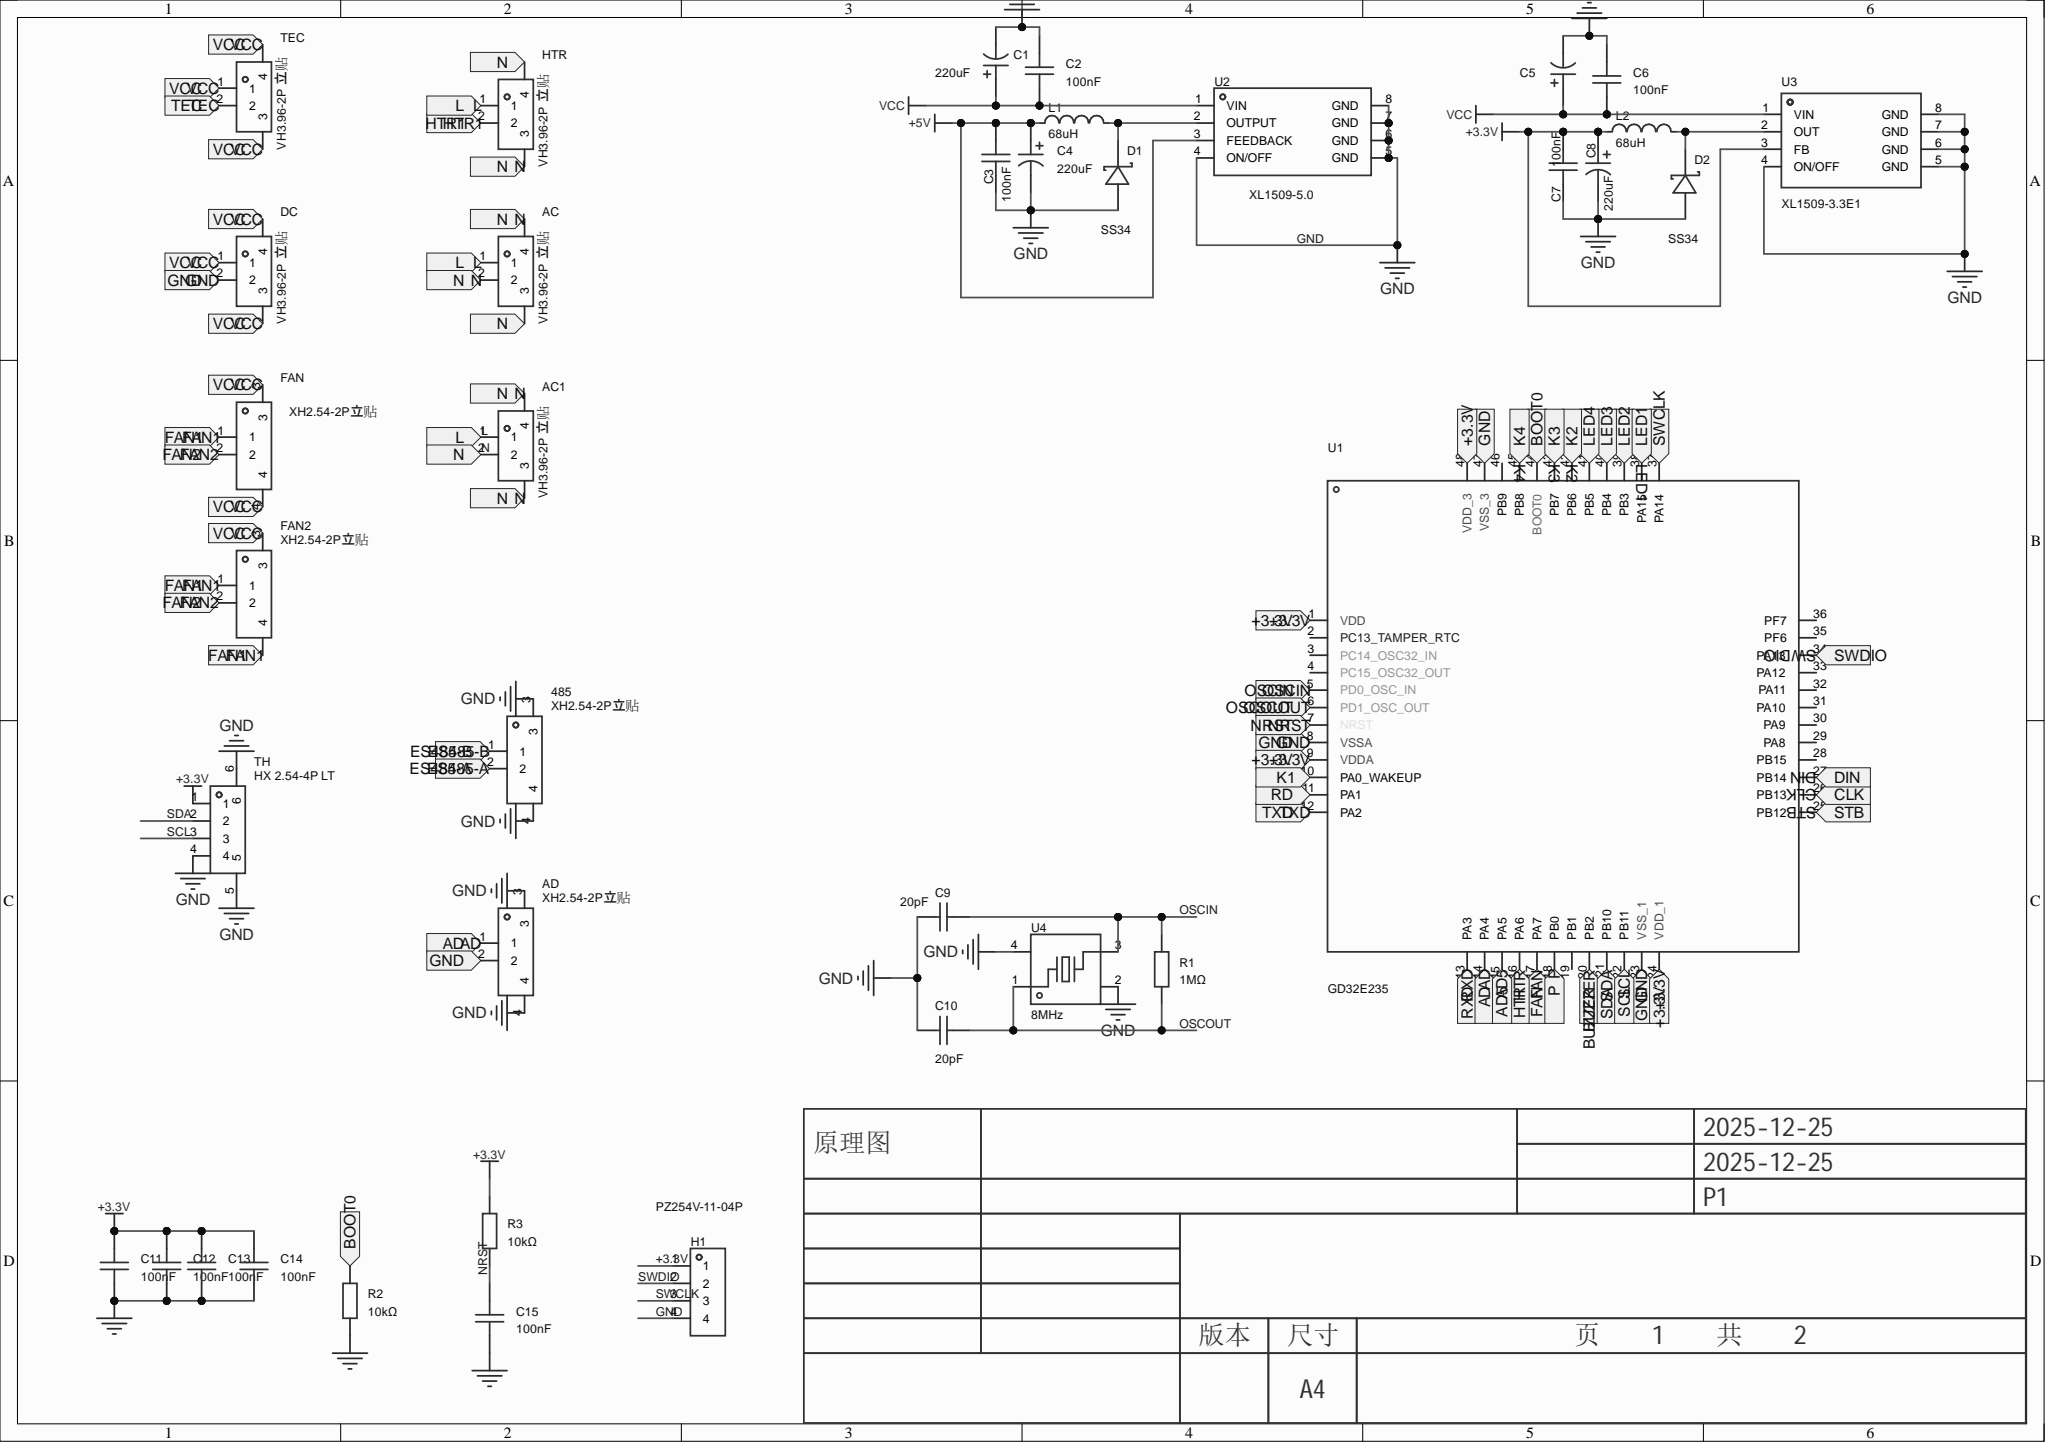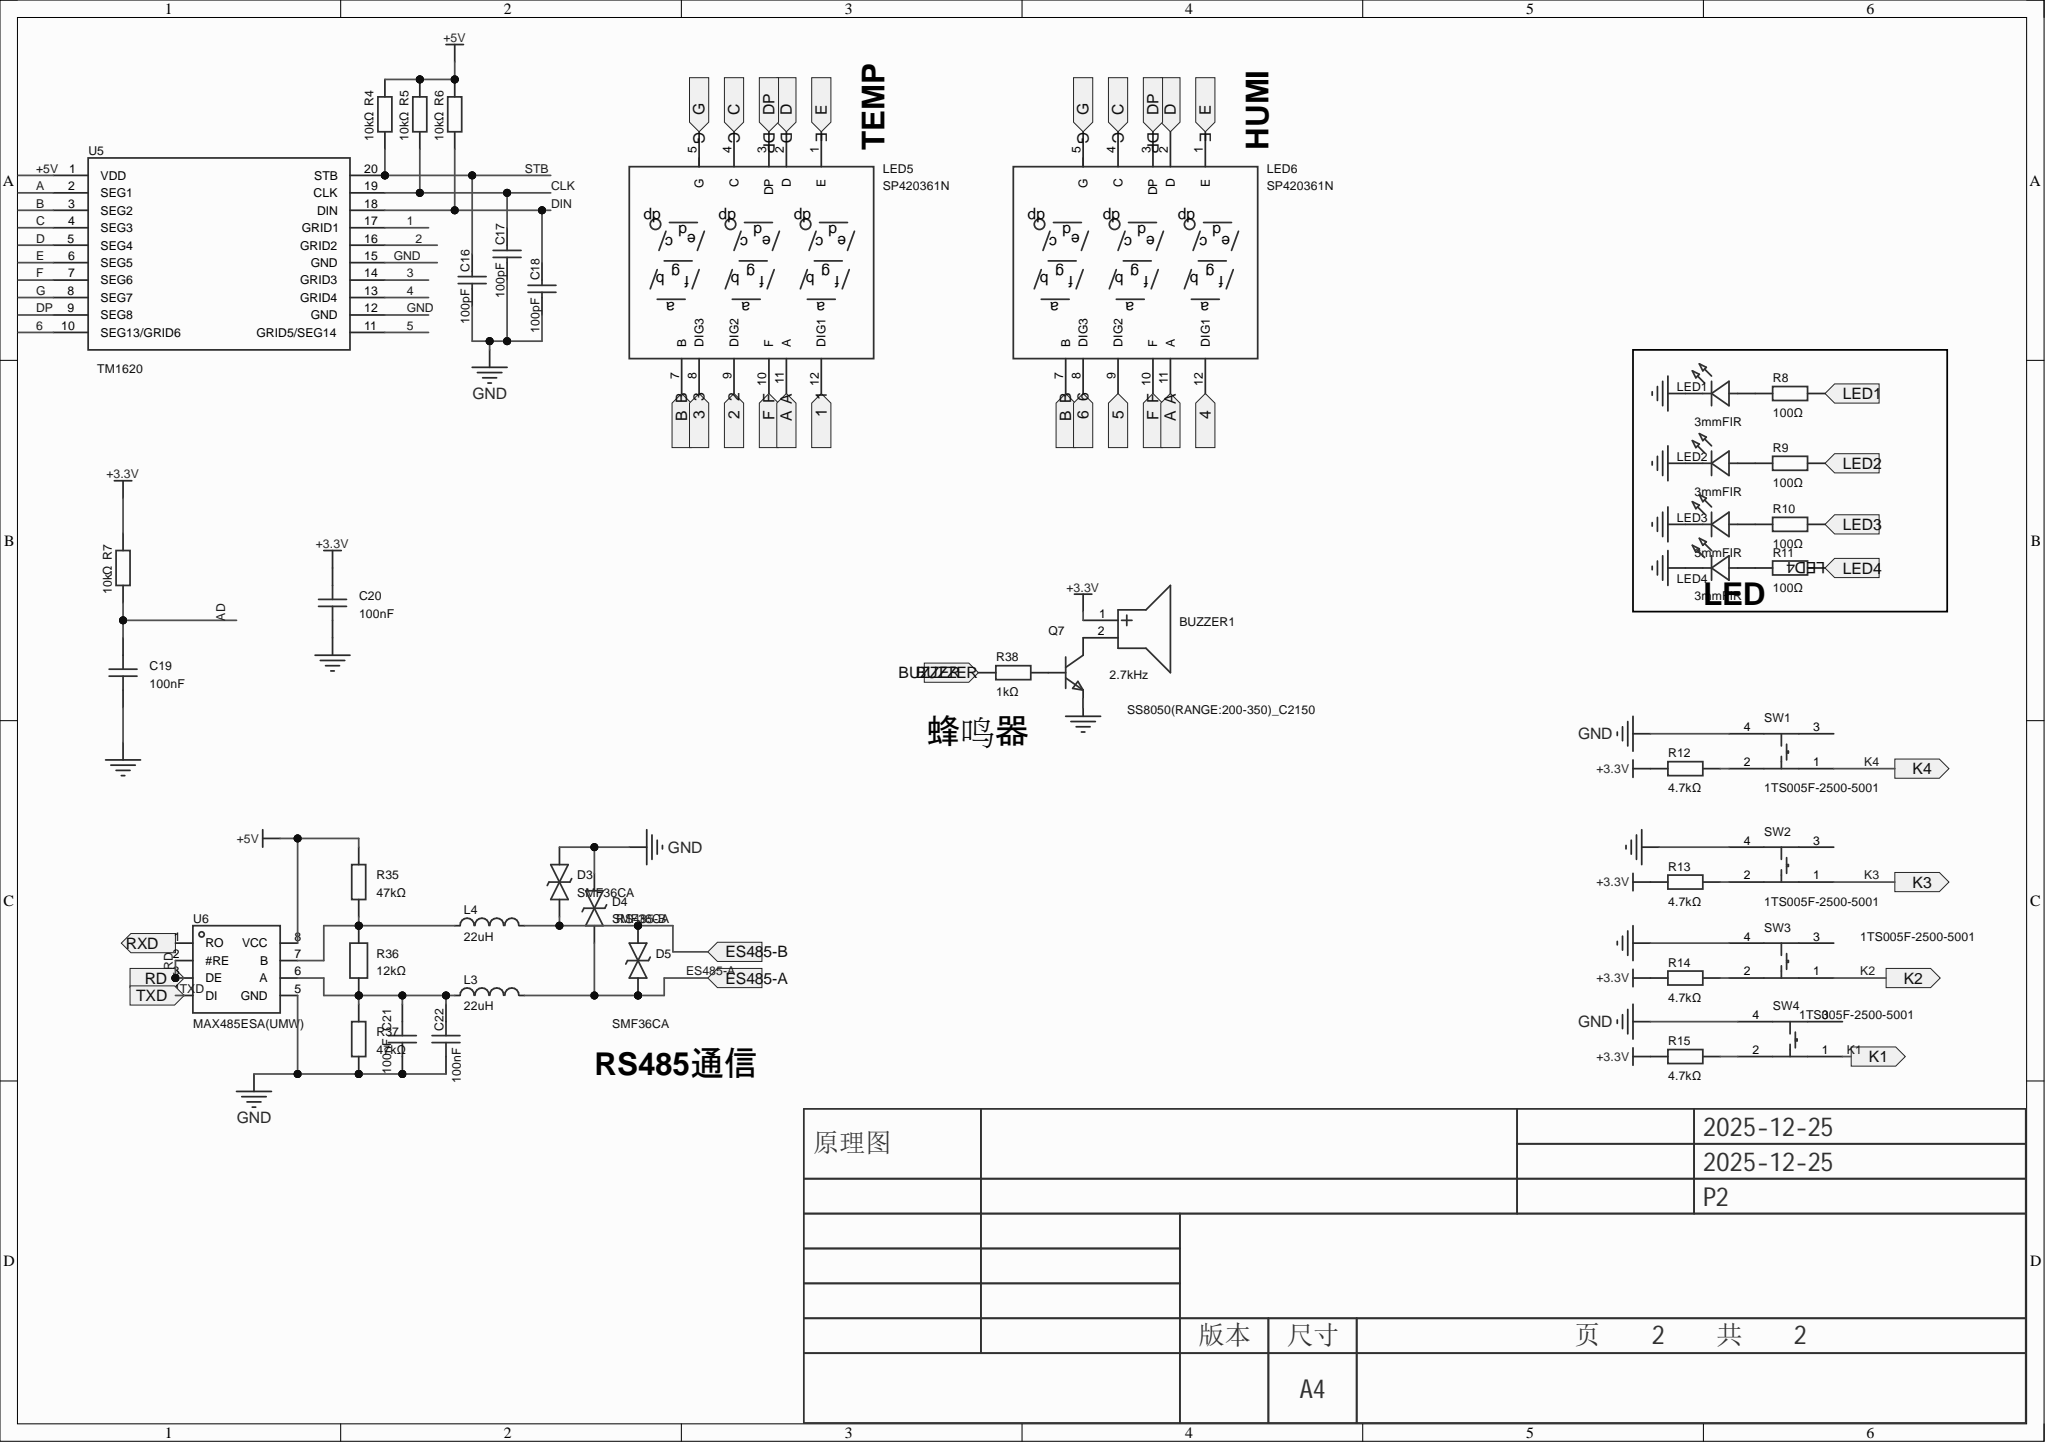Circuit board | Altium Designer | 106 parts | 82 nets
Bill of materials:
Comment,Description,Designator,Footprint,LibRef,Quantity
"XH2.54-2P立贴","","485, AD, FAN, FAN2","CONN-SMD_2P_A2501WV-S","XH2.54-2P立贴","4"
"VH3.96-2P 立贴","","AC, AC1, DC, HTR, TEC","CONN-SMD_2P-P3.96_HCTL_HC-VH-2ALT","VH3.96-2P 立贴","5"
"2.7kHz","驱动方式:有源(内含驱动线路);频率:2.7kHz;声压(SPL):80dB;","BUZZER1","BUZ-SMD_L9.6-W9.6-LS10.0-R","YS-SBZ9650DYB05","1"
"220uF","容值:220uF;精度:±20%;额定电压:35V;纹波电流:190mA@120Hz;","C1, C4, C8","CAP-SMD_BD6.3-L6.6-W6.6-FD","JVJ35V220M6x8","3"
"100nF","容值:100nF;精度:±10%;额定电压:50V;温度系数:X7R;","C2, C3, C6, C7, C11, C12, C13, C14, C15, C19, C20, C21, C22","C0805","FCC0805B104K500DT","13"
"C5","容值:220uF;精度:±20%;额定电压:35V;纹波电流:190mA@120Hz;","C5","CAP-SMD_BD6.3-L6.6-W6.6-FD","JVJ35V220M6x8","1"
"20pF","容值:20pF;精度:±5%;额定电压:50V;温度系数:C0G;","C9, C10","C0805","CL21C200JBANNNC","2"
"100pF","容值:100pF;精度:±5%;额定电压:50V;温度系数:C0G;","C16, C17, C18","C0805","CL21C101JBANNNC","3"
"10nF","容值:10nF;精度:±10%;额定电压:50V;温度系数:X7R;","C23","C1210","1210B103K500NT","1"
"SS34","二极管配置:独立式;正向压降(Vf):550mV@3A;直流反向耐压(Vr):40V;整流电流:3A;","D1, D2","SMA_L4.3-W2.6-LS5.2-RD","SS34_C8678","2"
"SMF36CA","极性:双向;反向截止电压(Vrwm):36V;钳位电压:58.1V;峰值脉冲电流(Ipp):3.5A;峰值脉冲功率(Ppp):200W@10/1000us;击穿电压:40V;","D3, D4, D5","SOD-123_L2.7-W1.8-LS3.7-BI","SMF36CA_C435502","3"
"PZ254V-11-04P","插针结构:1x4P;间距:2.54mm;行距:-;圆针/方针:方针;安装方式:直插;排数:单排;总PIN位数:4P;额定电流:3A;额定电压:250V;配合针长度:6mm;塑高:2.5mm;端接针长度:3mm;触头材质:-;工作温度:-40℃~+105℃;颜色:黑色;","H1","HDR-TH_4P-P2.54-V-M","PZ254V-11-04P","1"
"68uH","电感值:68uH;精度:±20%;额定电流:1.5A;饱和电流(Isat):2A;类型:-;","L1, L2","IND-SMD_L7.1-W6.6_H5.0","PSPMAA0605H-680M-IGF","2"
"22uH","","L3, L4","L1206","SCL3216T220KSP","2"
"3mmFIR","","LED1, LED2, LED3, LED4","LED-TH_BD3.0-P2.54-FD","3mmFIR","4"
"SP420361N","和我买的30V测电器的数码管尺寸一样，数码管位数:3位;发光颜色:红色;LED极性:共阴极;数字/字母大小(英寸):0.36;","LED5, LED6","LED-SEG-TH_SP420361N","EPHB_SP420361N 0.36英寸3位红色数码管","2"
"HYG140N10","类型:1个N沟道;漏源电压(Vdss):100V;连续漏极电流(Id):45A;导通电阻(RDS(on)@Vgs,Id):-;功率(Pd):3W;阈值电压(Vgs(th)@Id):2.5V@250uA;","Q1","TO-252-3_L6.6-W6.1-P4.58-LS10.1-BR","NCE0140K2-VB","1"
"SS8050(RANGE:200-350)","晶体管类型:NPN;集电极电流(Ic):1.5A;集射极击穿电压(Vceo):25V;功率(Pd):300mW;直流电流增益(hFE@Ic,Vce):200@800mA,1V;","Q2, Q3, Q6, Q7","SOT-23-3_L2.9-W1.3-P1.90-LS2.4-BR","SS8050(RANGE:200-350)_C2150","4"
"HYG025N06LS1B","","Q4","TO-263-2_L10.2-W8.7-P5.08-LS15.1-BR","HYG025N06LS1B","1"
"BTA216B-600D-JSM","保持电流(Ih):25mA;断态峰值电压(Vdrm):600V;门极触发电流(Igt):50mA;","Q8","TO-263-3_L10.2-W9.2-P5.08-LS15.4-BR","BTA216B-600D-JSM","1"
"1MΩ","","R1","R0805","0805W8F1004T5E","1"
"10kΩ","","R2, R3, R4, R5, R6, R7, R23, R27","R0805","0805W8F1002T5E_C17414","8"
"100Ω","","R8, R9, R10, R11","R0805","0805W8F1000T5E","4"
"4.7kΩ","","R12, R13, R14, R15, R20, R25","R0805","0805W8F4701T5E","6"
"24kΩ","","R16","R0805","0805W8F2402T5E","1"
"1kΩ","","R17, R18, R21, R24, R38","R0805","0805W8F1001T5E","5"
"5mΩ","","R19","R2010","WSL2010R0100FEA18","1"
"10","","R22, R26","R0805","Res_0805","2"
"1K","","R28","R0805","Res_0805","1"
"10K","","R29, R30","R0805","Res_0805","2"
"51Ω","","R31","R0204","MMA02040C5109FB300","1"
"150Ω","","R32","R0204","MMA02040E1500BB100","1"
"120Ω","","R33","R0204","CSR0204FTDV1200","1"
"47kΩ","","R35, R37","R0805","0805W8F4702T5E","2"
"12kΩ","","R36","R0805","FRC0805F1202TS","1"
"1TS005F-2500-5001","电路结构:单刀单掷;按钮形状:圆形按钮;作用力:2.5N;安装方式:立贴;开关长度:6mm;开关宽度:6mm;开关高度:5mm;带支架:不带支架;触点电流:50mA;额定电压:12V;带灯:无;工作寿命:7万次;","SW1, SW2, SW3, SW4","SW-SMD_4P-L6.0-W6.0-P4.50-LS9.0-H2.5","1TS005F-2500-5001","4"
"HX 2.54-4P LT","插针结构:1x4P;间距:2.54mm;安装方式:立贴;参考系列:XH;总PIN数:4P;排数:1;每排PIN数:4;行距:-;额定电流:3A;触头材质:黄铜;触头镀层:锡;工作温度:-25℃~+85℃;","TH","CONN-SMD_4P-P2.50_HX-2.54-4P-LT","HX 2.54-4P LT","1"
"GD32E235","CPU内核:ARM-M23;CPU最大主频:78MHz;应用领域:-;","U1","TQFP-48_L7.0-W7.0-P0.50-LS9.0-BL","GD32E235CBT61","1"
"XL1509-5.0","功能类型:降压型;输出类型:固定;工作电压:4.5V~40V;输出电压:5V;输出电流:2A;","U2","SOIC-8_L4.9-W3.9-P1.27-LS6.0-TR","XL1509-5.0","1"
"XL1509-3.3E1","功能类型:降压型;工作电压:4.5V~40V;输出电压:3.3V;输出电流:2A;输出类型:固定;","U3","SOP-8_L4.9-W3.9-P1.27-LS6.0-BL","XL1509-3.3E1","1"
"8MHz","晶振类型:贴片晶振;频率:8MHz;常温频差:±10ppm;负载电容:20pF;频率稳定度:±20ppm;","U4","CRYSTAL-SMD_4P-L3.2-W2.5-BL","XL2SI-111-8M","1"
"TM1620","显示模式（8段×6位~10段x4位）的LED 驱动IC","U5","SOIC-20_L13.0-W7.6-P1.27-LS10.3-BL","TM1620","1"
"MAX485ESA(UMW)","","U6","SOP-8_L5.0-W4.0-P1.27-LS6.0-BL","MAX485ESA(UMW)","1"
"LMV321","放大器数:单路;轨到轨:-;增益带宽积(GBP):1MHz;输入失调电压(Vos):9mV;压摆率(SR):400V/ms;输入偏置电流(Ib):45nA;","U7","SOT-23-5_L3.0-W1.7-P0.95-LS2.8-BR","LMV321","1"
"ELM3083(TA)-V","正向电压:1.5V;正向电流:60mA;负载电压:800V;静态dv/dt:1000V/us;","U8","SOP-4_L4.4-W4.0-P2.54-LS7.0-TL","ELM3083(TA)-V","1"
Netlist (Protel format):
[
485
CONN-SMD_2P_A2501WV-S
XH2.54-2P立贴



]
[
AC
CONN-SMD_2P-P3.96_HCTL_HC-VH-2ALT
VH3.96-2P 立贴



]
[
AC1
CONN-SMD_2P-P3.96_HCTL_HC-VH-2ALT
VH3.96-2P 立贴



]
[
AD
CONN-SMD_2P_A2501WV-S
XH2.54-2P立贴



]
[
BUZZER1
BUZ-SMD_L9.6-W9.6-LS10.0-R
2.7kHz



]
[
C1
CAP-SMD_BD6.3-L6.6-W6.6-FD
220uF



]
[
C2
C0805
100nF



]
[
C3
C0805
100nF



]
[
C4
CAP-SMD_BD6.3-L6.6-W6.6-FD
220uF



]
[
C5
CAP-SMD_BD6.3-L6.6-W6.6-FD
C5



]
[
C6
C0805
100nF



]
[
C7
C0805
100nF



]
[
C8
CAP-SMD_BD6.3-L6.6-W6.6-FD
220uF



]
[
C9
C0805
20pF



]
[
C10
C0805
20pF



]
[
C11
C0805
100nF



]
[
C12
C0805
100nF



]
[
C13
C0805
100nF



]
[
C14
C0805
100nF



]
[
C15
C0805
100nF



]
[
C16
C0805
100pF



]
[
C17
C0805
100pF



]
[
C18
C0805
100pF



]
[
C19
C0805
100nF



]
[
C20
C0805
100nF



]
[
C21
C0805
100nF



]
[
C22
C0805
100nF



]
[
C23
C1210
10nF



]
[
D1
SMA_L4.3-W2.6-LS5.2-RD
SS34



]
[
D2
SMA_L4.3-W2.6-LS5.2-RD
SS34



]
[
D3
SOD-123_L2.7-W1.8-LS3.7-BI
SMF36CA



]
[
D4
SOD-123_L2.7-W1.8-LS3.7-BI
SMF36CA



]
[
D5
SOD-123_L2.7-W1.8-LS3.7-BI
SMF36CA



]
[
DC
CONN-SMD_2P-P3.96_HCTL_HC-VH-2ALT
VH3.96-2P 立贴



]
[
FAN
CONN-SMD_2P_A2501WV-S
XH2.54-2P立贴



]
[
FAN2
CONN-SMD_2P_A2501WV-S
XH2.54-2P立贴



]
[
H1
HDR-TH_4P-P2.54-V-M
PZ254V-11-04P



]
[
HTR
CONN-SMD_2P-P3.96_HCTL_HC-VH-2ALT
VH3.96-2P 立贴



]
[
L1
IND-SMD_L7.1-W6.6_H5.0
68uH



]
[
L2
IND-SMD_L7.1-W6.6_H5.0
68uH



]
[
L3
L1206
22uH



]
[
L4
L1206
22uH



]
[
LED1
LED-TH_BD3.0-P2.54-FD
3mmFIR



]
[
LED2
LED-TH_BD3.0-P2.54-FD
3mmFIR



]
[
LED3
LED-TH_BD3.0-P2.54-FD
3mmFIR



]
[
LED4
LED-TH_BD3.0-P2.54-FD
3mmFIR



]
[
LED5
LED-SEG-TH_SP420361N
SP420361N



]
[
LED6
LED-SEG-TH_SP420361N
SP420361N



]
[
Q1
TO-252-3_L6.6-W6.1-P4.58-LS10.1-BR
HYG140N10



]
[
Q2
SOT-23-3_L2.9-W1.3-P1.90-LS2.4-BR
SS8050(RANGE:200-350)



]
[
Q3
SOT-23-3_L2.9-W1.3-P1.90-LS2.4-BR
SS8050(RANGE:200-350)



]
[
Q4
TO-263-2_L10.2-W8.7-P5.08-LS15.1-BR
HYG025N06LS1B



]
[
Q6
SOT-23-3_L2.9-W1.3-P1.90-LS2.4-BR
SS8050(RANGE:200-350)



]
[
Q7
SOT-23-3_L2.9-W1.3-P1.90-LS2.4-BR
SS8050(RANGE:200-350)



]
[
Q8
TO-263-3_L10.2-W9.2-P5.08-LS15.4-BR
BTA216B-600D-JSM



]
[
R1
R0805
1MΩ



]
[
R2
R0805
10kΩ



]
[
R3
R0805
10kΩ



]
[
R4
R0805
10kΩ



]
[
R5
R0805
10kΩ



]
[
R6
R0805
10kΩ



]
[
R7
R0805
10kΩ



]
[
R8
R0805
100Ω



]
[
R9
R0805
100Ω



]
[
R10
R0805
100Ω



]
[
R11
R0805
100Ω



]
[
R12
R0805
4.7kΩ



]
[
R13
R0805
4.7kΩ



]
[
R14
R0805
4.7kΩ



]
[
R15
R0805
4.7kΩ



]
[
R16
R0805
24kΩ



]
[
R17
R0805
1kΩ



]
[
R18
R0805
1kΩ



]
[
R19
R2010
5mΩ



]
[
R20
R0805
4.7kΩ



]
[
R21
R0805
1kΩ



]
[
R22
R0805
10



]
[
R23
R0805
10kΩ



]
[
R24
R0805
1kΩ



]
[
R25
R0805
4.7kΩ



]
[
R26
R0805
10



]
[
R27
R0805
10kΩ



]
[
R28
R0805
1K



]
[
R29
R0805
10K



]
[
R30
R0805
10K



]
[
R31
R0204
51Ω



]
[
R32
R0204
150Ω



]
[
R33
R0204
120Ω



]
[
R35
R0805
47kΩ



]
[
R36
R0805
12kΩ



]
[
R37
R0805
47kΩ



]
[
R38
R0805
1kΩ



]
[
SW1
SW-SMD_4P-L6.0-W6.0-P4.50-LS9.0-H2.5
1TS005F-2500-5001



]
[
SW2
SW-SMD_4P-L6.0-W6.0-P4.50-LS9.0-H2.5
1TS005F-2500-5001



]
[
SW3
SW-SMD_4P-L6.0-W6.0-P4.50-LS9.0-H2.5
1TS005F-2500-5001



]
[
SW4
SW-SMD_4P-L6.0-W6.0-P4.50-LS9.0-H2.5
1TS005F-2500-5001



]
[
TEC
CONN-SMD_2P-P3.96_HCTL_HC-VH-2ALT
VH3.96-2P 立贴



]
[
TH
CONN-SMD_4P-P2.50_HX-2.54-4P-LT
HX 2.54-4P LT



]
[
U1
TQFP-48_L7.0-W7.0-P0.50-LS9.0-BL
GD32E235



]
[
U2
SOIC-8_L4.9-W3.9-P1.27-LS6.0-TR
XL1509-5.0



]
[
U3
SOP-8_L4.9-W3.9-P1.27-LS6.0-BL
XL1509-3.3E1



]
[
U4
CRYSTAL-SMD_4P-L3.2-W2.5-BL
8MHz



]
[
U5
SOIC-20_L13.0-W7.6-P1.27-LS10.3-BL
TM1620



]
[
U6
SOP-8_L5.0-W4.0-P1.27-LS6.0-BL
MAX485ESA(UMW)



]
[
U7
SOT-23-5_L3.0-W1.7-P0.95-LS2.8-BR
LMV321



]
[
U8
SOP-4_L4.4-W4.0-P2.54-LS7.0-TL
ELM3083(TA)-V



]
(
VCC
C1-1
C2-1
C5-1
C6-1
DC-1
DC-3
DC-4
FAN-3
FAN-4
FAN2-3
R17-2
R19-2
R30-2
TEC-1
TEC-3
TEC-4
U2-1
U3-1
)
(
TXD
U1-12
U6-4
)
(
SWDIO
H1-2
U1-34
)
(
STB
C16-2
R4-1
U5-20
)
(
SDA
TH-2
U1-21
)
(
SCL
TH-3
U1-22
)
(
RXD
U1-13
U6-1
)
(
RD
U1-11
U6-2
U6-3
)
(
PL
Q4-4
TEC-2
)
(
P
R24-1
U1-18
)
(
OSCOUT
C10-2
R1-1
U1-6
U4-1
)
(
OSCIN
C9-2
R1-2
U1-5
U4-3
)
(
NRST
C15-2
R3-1
U1-7
)
(
NetR31_1
R31-1
U8-3
)
(
NetR30_1
R30-1
U8-1
)
(
NetR18_1
R18-1
U7-3
)
(
NetR16_1
R16-1
R17-1
U7-1
)
(
NetR15_1
R15-1
SW4-2
)
(
NetR14_1
R14-1
SW3-2
)
(
NetR13_1
R13-1
SW2-2
)
(
NetR12_1
R12-1
SW1-2
)
(
NetR10_2
R10-2
U1-40
)
(
NetR9_2
R9-2
U1-39
)
(
NetR2_2
R2-2
U1-44
)
(
NetQ8_3
Q8-3
R31-2
R32-1
)
(
NetQ7_1
Q7-1
R38-2
)
(
NetQ6_3
Q6-3
U8-2
)
(
NetQ6_1
Q6-1
R28-2
R29-1
)
(
NetQ4_1
Q4-1
R26-2
R27-2
)
(
NetQ3_3
Q3-3
R25-2
)
(
NetQ3_2
Q3-2
R26-1
)
(
NetQ3_1
Q3-1
R24-2
)
(
NetQ2_3
Q2-3
R20-2
)
(
NetQ2_2
Q2-2
R22-1
)
(
NetQ2_1
Q2-1
R21-2
)
(
NetQ1_1
Q1-1
R22-2
R23-2
)
(
NetLED4_1
LED4-1
R11-1
)
(
NetLED3_1
LED3-1
R10-1
)
(
NetLED2_1
LED2-1
R9-1
)
(
NetLED1_1
LED1-1
R8-1
)
(
NetL4_1
L4-1
R35-1
R36-2
U6-7
)
(
NetD2_1
D2-1
L2-2
U3-2
)
(
NetD1_1
D1-1
L1-2
U2-2
)
(
NetC23_2
C23-2
R33-1
)
(
NetC21_2
C21-2
C22-2
L3-1
R36-1
R37-2
U6-6
)
(
NetBUZZER1_2
BUZZER1-2
Q7-3
)
(
N
AC-2
AC-3
AC-4
AC1-2
AC1-3
AC1-4
C23-1
HTR-3
HTR-4
Q8-1
R32-2
)
(
LED4
R11-2
U1-41
)
(
LED1
R8-2
U1-38
)
(
L
AC-1
AC1-1
HTR-1
)
(
K4
SW1-1
U1-45
)
(
K3
SW2-1
U1-43
)
(
K2
SW3-1
U1-42
)
(
K1
SW4-1
U1-10
)
(
HTR1
HTR-2
Q8-2
R33-2
U8-4
)
(
HTR
R28-1
U1-16
)
(
GND
485-3
485-4
AD-2
AD-3
AD-4
C1-2
C2-2
C3-1
C4-2
C5-2
C6-2
C7-1
C8-2
C9-1
C10-1
C11-1
C12-1
C13-1
C14-1
C15-1
C16-1
C17-1
C18-1
C19-1
C20-1
C21-1
C22-1
D1-2
D2-2
D3-2
D4-2
DC-2
H1-4
LED1-2
LED2-2
LED3-2
LED4-2
Q1-2
Q4-3
Q6-2
Q7-2
R2-1
R16-2
R23-1
R27-1
R29-2
R37-1
SW1-4
SW2-4
SW3-4
SW4-4
TH-4
TH-5
TH-6
U1-8
U1-23
U1-47
U2-4
U2-5
U2-6
U2-7
U2-8
U3-4
U3-5
U3-6
U3-7
U3-8
U4-2
U4-4
U5-12
U5-15
U6-5
U7-2
)
(
G
LED5-5
LED6-5
U5-8
)
(
FAN2
FAN-2
FAN2-2
R18-2
R19-1
)
(
FAN1
FAN-1
FAN2-1
FAN2-4
Q1-3
)
(
FAN
R21-1
U1-17
)
(
F
LED5-10
LED6-10
U5-7
)
(
ES485-B
485-1
D3-1
D5-2
L4-2
)
(
ES485-A
485-2
D4-1
D5-1
L3-2
)
(
E
LED5-1
LED6-1
U5-6
)
(
DP
LED5-3
LED6-3
U5-9
)
(
DIN
C18-2
R6-1
U5-18
)
(
D
LED5-2
LED6-2
U5-5
)
(
CLK
C17-2
R5-1
U5-19
)
(
C
LED5-4
LED6-4
U5-4
)
(
BUZZER
R38-1
U1-20
)
(
B
LED5-7
LED6-7
U5-3
)
(
AD5
U1-15
U7-4
)
(
AD
AD-1
U1-14
)
(
AD
C19-2
R7-1
)
(
A
LED5-11
LED6-11
U5-2
)
(
+5V
C3-2
C4-1
L1-1
R4-2
R5-2
R6-2
R20-1
R25-1
R35-2
U2-3
U5-1
U6-8
)
(
+3.3V
BUZZER1-1
C7-2
C8-1
C11-2
C12-2
C13-2
C14-2
C20-2
H1-1
L2-1
R3-2
R7-2
R12-2
R13-2
R14-2
R15-2
TH-1
U1-1
U1-9
U1-24
U1-48
U3-3
U7-5
)
(
6
LED6-8
U5-10
)
(
3
LED5-8
U5-14
)
(
2
LED5-9
U5-16
)
(
1
LED5-12
U5-17
)